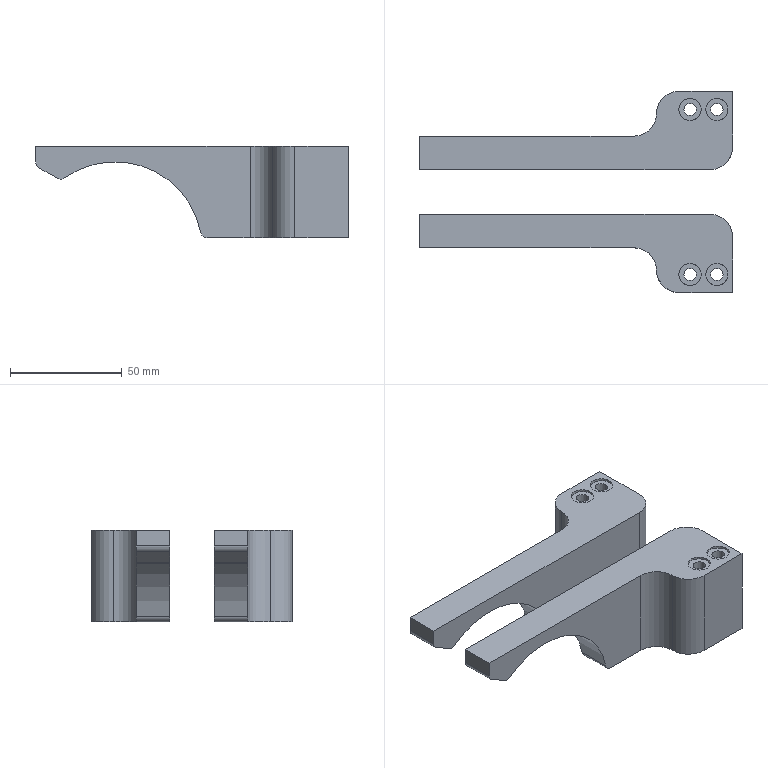NC program | NX | posted with a generic post | part box 140 x 90 x 41 mm
Lines 43 to 1092 of 28919:
(ADAPTIVE_MILLING , TOOL : D12C)
N72 T12 M6
N74 G54
N76 G17 G0 G90 X84.203 Y-7.467 S9500 M3
N78 G43 Z30. H12
N80 Z-17.5
N82 G94 G1 Z-20.5 F1000.
N84 X82.519 Y-6.874 F3000.
N86 G3 X81.036 Y-7.467 R1.218
N88 X80.297 Y-10.773 R9.606
N90 X80.002 Y-19.69 R131.632
N92 G2 X76.897 Y-24.615 R7.1
N94 X70.842 Y-26.888 R14.21
N96 X61.567 Y-27.447 R65.362
N98 G1 X60.442 Y-27.459
N100 X59.092 Y-27.468
N102 X57.517 Y-27.475
N104 X55.267 Y-27.481
N106 X51.817 Y-27.485
N108 X44.242 Y-27.486
N110 X-71.708 Y-27.483
N112 X-71.783
N114 X-71.858 Y-27.481
N116 X-72.007 Y-27.473
N118 X-72.082 Y-27.468
N120 G2 X-77.095 Y-24.379 R7.057
N122 X-79.394 Y-18.256 R14.245
N124 X-79.942 Y-9.431 R62.966
N126 G1 X-79.955 Y-8.306
N128 X-79.965 Y-7.106
N130 X-79.973 Y-5.606
N132 X-79.979 Y-3.581
N134 X-79.984 Y-0.656
N136 X-79.986 Y4.744
N138 G2 X-79.956 Y19.743 R731.547
N140 X-76.746 Y24.687 R7.169
N142 X-70.521 Y26.929 R14.668
N144 X-61.843 Y27.44 R66.663
N146 G1 X-60.793 Y27.451
N148 X-59.518 Y27.462
N150 X-57.943 Y27.47
N152 X-55.918 Y27.476
N154 X-52.918 Y27.48
N156 X-47.218 Y27.483
N158 X44.582 Y27.484
N160 X45.332 Y27.487
N162 X46.232 Y27.488
N164 X46.682
N166 X47.507 Y27.491
N168 X48.707 Y27.49
N170 X49.382 Y27.492
N172 X50.582
N174 X51.557 Y27.494
N176 X52.307
N178 X53.657 Y27.495
N180 X54.107 Y27.496
N182 X54.932 Y27.494
N184 X56.057 Y27.496
N186 X56.807 Y27.495
N188 X58.007 Y27.496
N190 X58.907 Y27.494
N192 X59.657 Y27.495
N194 X60.932 Y27.493
N196 X61.382
N198 X62.207 Y27.495
N200 X63.332 Y27.493
N202 X64.082 Y27.495
N204 X65.357 Y27.493
N206 G2 X72.33 Y27.454 R153.694
N208 X77.24 Y24.187 R7.229
N210 X79.455 Y17.873 R14.887
N212 X79.951 Y8.518 R73.908
N214 X79.941 Y-4.456 R389.185
N216 G3 X79.221 Y-12.674 R226.057
N218 G2 X79.02 Y-17.017 R73.793
N220 X74.352 Y-23.663 R9.401
N222 X67.403 Y-25.901 R18.272
N224 X56.849 Y-26.44 R86.916
N226 G1 X55.574 Y-26.45
N228 X53.999 Y-26.459
N230 X51.974 Y-26.466
N232 X49.124 Y-26.471
N234 X44.399 Y-26.474
N236 X28.949 Y-26.475
N238 X-68.326 Y-26.472
N240 X-68.476 Y-26.471
N242 X-68.701 Y-26.463
N244 X-68.851 Y-26.456
N246 G2 X-75.934 Y-22.12 R9.114
N248 X-78.359 Y-15.085 R17.36
N250 X-78.923 Y-5.659 R73.598
N252 G1 X-78.936 Y-4.609
N254 X-78.947 Y-3.409
N256 X-78.957 Y-1.834
N258 X-78.964 Y0.041
N260 X-78.97 Y2.591
N262 X-78.974 Y6.491
N264 G2 X-78.94 Y16.615 R387.568
N266 X-74.588 Y23.454 R9.146
N268 X-67.547 Y25.863 R17.473
N270 X-57.67 Y26.426 R77.667
N272 G1 X-56.695 Y26.437
N274 X-55.345 Y26.448
N276 X-53.695 Y26.456
N278 X-51.595 Y26.463
N280 X-48.67 Y26.468
N282 X-43.57 Y26.471
N284 X-21.37 Y26.472
N286 X41.18
N288 X42.305 Y26.479
N290 X43.355
N292 X44.33 Y26.484
N294 X45.605 Y26.483
N296 X46.355 Y26.486
N298 X47.33 Y26.487
N300 X47.705
N302 X48.605 Y26.49
N304 X49.73 Y26.489
N306 X50.78 Y26.493
N308 X51.905 Y26.492
N310 X52.88 Y26.494
N312 X53.78 Y26.493
N314 X54.905 Y26.496
N316 X55.955 Y26.494
N318 X57.005 Y26.496
N320 X58.13 Y26.493
N322 X59.255 Y26.495
N324 X60.08 Y26.494
N326 X60.98 Y26.495
N328 X61.355
N330 X62.18 Y26.494
N332 G2 X69.154 Y26.454 R208.519
N334 X75.977 Y22.075 R9.16
N336 X78.357 Y15.101 R17.532
N338 X78.932 Y4.775 R79.803
N340 X78.813 Y-4.596 R113.198
N342 G3 X78.147 Y-14.323 R772.732
N344 G2 X72.411 Y-22.625 R10.832
N346 X64.914 Y-24.877 R20.889
N348 X54.359 Y-25.419 R93.029
N350 G1 X53.159 Y-25.431
N352 X51.734 Y-25.441
N354 X49.934 Y-25.449
N356 X47.684 Y-25.456
N358 X44.384 Y-25.46
N360 X38.609 Y-25.463
N362 X-0.091 Y-25.462
N364 X-65.491 Y-25.46
N366 X-65.791 Y-25.457
N368 X-66.016 Y-25.451
N370 X-66.241 Y-25.441
N372 G2 X-72.322 Y-23.181 R10.254
N374 X-75.927 Y-19.196 R6.416
N376 X-77.65 Y-10.166 R32.289
N378 X-77.954 Y3.703 R225.891
N380 X-77.925 Y14.052 R391.638
N382 X-72.524 Y22.469 R10.509
N384 X-64.844 Y24.866 R20.314
N386 X-54.44 Y25.413 R90.966
N388 G1 X-53.24 Y25.425
N390 X-51.815 Y25.436
N392 X-50.09 Y25.445
N394 X-47.84 Y25.452
N396 X-44.69 Y25.457
N398 X-39.29 Y25.459
N400 X-15.59 Y25.46
N402 X37.81 Y25.461
N404 X38.485 Y25.464
N406 X39.835 Y25.468
N408 X40.51 Y25.469
N410 X41.26 Y25.473
N412 X42.235 Y25.474
N414 X42.685 Y25.475
N416 X43.36 Y25.478
N418 X44.41 Y25.479
N420 X45.16 Y25.482
N422 X45.76 Y25.484
N424 X46.585
N426 X47.785 Y25.488
N428 X48.91 Y25.487
N430 X49.735 Y25.49
N432 X50.785
N434 X51.235
N436 X51.985 Y25.492
N438 X52.96 Y25.491
N440 X53.485 Y25.492
N442 X54.085 Y25.493
N444 X55.285 Y25.492
N446 X56.185 Y25.494
N448 X57.085 Y25.493
N450 G2 X66.609 Y25.447 R290.876
N452 X72.375 Y23.162 R10.225
N454 X75.927 Y19.196 R6.438
N456 X77.619 Y10.54 R31.649
N458 X77.503 Y-8.492 R129.148
N460 X76.984 Y-13.709 R31.363
N462 X70.481 Y-21.7 R12.003
N464 X62.42 Y-23.899 R23.823
N466 X50.887 Y-24.414 R113.709
N468 G1 X49.462 Y-24.425
N470 X47.737 Y-24.434
N472 X45.562 Y-24.442
N474 X42.637 Y-24.447
N476 X37.987 Y-24.451
N478 X26.287 Y-24.452
N480 X-62.963 Y-24.449
N482 X-63.263 Y-24.446
N484 X-63.488 Y-24.442
N486 X-63.788 Y-24.434
N488 G2 X-68.052 Y-23.662 R14.863
N490 X-71.435 Y-23.472 R19.024
N492 G1 X-72.497 Y-23.101
N494 G2 X-75.564 Y-20.101 R6.355
N496 X-76.15 Y-16.64 R7.644
N498 X-76.933 Y3.513 R227.343
N500 X-76.896 Y11.987 R202.597
N502 X-70.759 Y21.434 R11.503
N504 X-62.836 Y23.82 R21.994
N506 X-51.607 Y24.401 R97.353
N508 G1 X-50.407 Y24.413
N510 X-48.907 Y24.424
N512 X-47.182 Y24.433
N514 X-45.007 Y24.439
N516 X-41.857 Y24.445
N518 X-36.757 Y24.448
N520 X-20.407 Y24.449
N522 X34.493
N524 X35.318 Y24.454
N526 X36.143 Y24.455
N528 X36.593 Y24.456
N530 X37.268 Y24.459
N532 X38.543 Y24.462
N534 X39.293 Y24.466
N536 X40.493 Y24.467
N538 X41.168 Y24.471
N540 X42.293 Y24.472
N542 X42.968 Y24.475
N544 X44.018 Y24.477
N546 X44.543 Y24.478
N548 X45.068 Y24.48
N550 X46.043 Y24.481
N552 X46.418
N554 X47.243 Y24.485
N556 X48.443
N558 X49.268 Y24.488
N560 X50.318 Y24.487
N562 X51.293 Y24.49
N564 X52.343 Y24.489
N566 X53.168 Y24.491
N568 X54.068
N570 X54.593
N572 G2 X64.416 Y24.436 R271.367
N574 X68.15 Y23.66 R15.7
N576 X71.435 Y23.472 R18.018
N578 G1 X72.497 Y23.101
N580 G3 X69.965 Y23.65 R7.108
N582 G1 X68.243
N584 G3 X51.898 Y23.888 R308.852
N586 G1 X50.923 Y23.885
N588 X49.648 Y23.887
N590 X48.823 Y23.884
N592 X47.698 Y23.885
N594 X46.348 Y23.88
N596 X45.748
N598 X44.023 Y23.874
N600 X43.423
N602 X42.898 Y23.872
N604 X41.698 Y23.871
N606 X40.873 Y23.868
N608 X40.198 Y23.866
N610 X39.673
N612 X39.148 Y23.864
N614 X37.573 Y23.862
N616 X37.123 Y23.859
N618 X34.123 Y23.857
N620 X23.473 Y23.855
N622 X4.198
N624 X3.898 Y23.854
N626 X-34.577
N628 X-34.952 Y23.852
N630 G3 X-56.176 Y23.685 R749.437
N632 X-65.4 Y22.633 R46.746
N634 X-72.288 Y19.16 R15.199
N636 X-75.81 Y12.195 R12.073
N638 X-76.301 Y3.819 R52.759
N640 X-76.15 Y-6.918 R367.334
N642 G1 Y-16.668
N644 Y-2.535
N646 X-76.146 Y-2.465
N648 G2 X-75.689 Y0.484 R38.279
N650 G3 X-75.204 Y7.816 R154.513
N652 G2 X-73.874 Y14.017 R18.203
N654 X-67.184 Y20.384 R12.794
N656 X-58.901 Y22.35 R26.994
N658 X-46.613 Y22.805 R141.362
N660 G1 X-44.963 Y22.816
N662 X-42.938 Y22.826
N664 X-41.288 Y22.832
N666 X-40.689 Y22.836
N668 X-39.414 Y22.841
N670 X-37.989 Y22.843
N672 X-37.314 Y22.846
N674 X-36.264 Y22.847
N676 X-35.739 Y22.848
N678 X-35.064 Y22.85
N680 X-34.239
N682 X-33.114 Y22.853
N684 X-32.139 Y22.851
N686 X-31.389 Y22.853
N688 X-30.264 Y22.852
N690 X-29.289 Y22.854
N692 X-28.539 Y22.853
N694 X-27.564 Y22.854
N696 X-26.814 Y22.853
N698 X-25.839 Y22.854
N700 X-24.864 Y22.852
N702 X-23.889 Y22.855
N704 X-22.839 Y22.853
N706 X-22.014 Y22.854
N708 X-20.814 Y22.853
N710 X-19.839 Y22.855
N712 X-18.864 Y22.853
N714 X-18.039 Y22.854
N716 X-16.914 Y22.853
N718 X-16.014 Y22.855
N720 X-14.964 Y22.853
N722 X-14.289 Y22.854
N724 X-13.314 Y22.853
N726 X-12.939 Y22.852
N728 X-12.189 Y22.854
N730 X-11.064 Y22.853
N732 X-10.089 Y22.855
N734 X-9.339 Y22.853
N736 X-8.289 Y22.855
N738 X-7.239 Y22.852
N740 X-6.414 Y22.854
N742 X-5.289 Y22.853
N744 X-4.464 Y22.854
N746 X-3.339 Y22.853
N748 X-2.439 Y22.854
N750 X-1.389 Y22.853
N752 X-0.714 Y22.854
N754 X0.261 Y22.853
N756 X0.636 Y22.852
N758 X1.686 Y22.855
N760 X2.436 Y22.854
N762 X3.411 Y22.855
N764 X4.161 Y22.854
N766 X5.136 Y22.856
N768 X6.111 Y22.854
N770 X7.086 Y22.856
N772 X7.911 Y22.854
N774 X9.036 Y22.856
N776 X9.936 Y22.855
N778 X10.911 Y22.856
N780 X11.811 Y22.855
N782 X12.861 Y22.857
N784 X13.536 Y22.855
N786 X14.511 Y22.857
N788 X14.886
N790 X15.636 Y22.856
N792 X16.761 Y22.857
N794 X17.736 Y22.855
N796 X18.486 Y22.856
N798 X19.536 Y22.855
N800 X20.586 Y22.857
N802 X21.486 Y22.855
N804 X22.386 Y22.856
N806 X23.286 Y22.855
N808 X24.261 Y22.857
N810 X25.311 Y22.854
N812 X26.211 Y22.856
N814 X27.336 Y22.854
N816 X28.161 Y22.856
N818 X29.136 Y22.855
N820 X29.961 Y22.856
N822 X30.936 Y22.855
N824 X31.686 Y22.857
N826 X32.736 Y22.856
N828 X33.486 Y22.857
N830 X34.536
N832 X35.286 Y22.859
N834 X36.411
N836 X37.536 Y22.864
N838 X38.286
N840 X39.261 Y22.867
N842 X40.011
N844 X40.911 Y22.87
N846 X40.986 Y22.872
N848 X41.061 Y22.878
N850 X41.135 Y22.89
N852 X43.425 Y23.44
N854 X43.523 Y23.455
N856 X45.975 Y23.648
N858 X46.025 Y23.65
N860 X67.85
N862 G3 X68.674 Y25.722 R1.201
N864 X68.042 Y26.058 Z-20.47 R1.681
N866 G1 X66.469 Y26.642 Z-20.4
N868 X64.309 Y27.434
N870 X64.031 Y27.468
N872 X43.835 Y27.566
N874 G3 X42.658 Y26.628 R1.208
N876 G1 X42.597 Y26.355
N878 X42.075 Y24.013 Z-20.5
N880 G2 X41.641 Y23.15 R1.418
N882 X41.135 Y22.89 R1.334
N884 X36.953 Y22.36 R16.121
N886 X15.504 Y22.256 R921.472
N888 G1 X13.854 Y22.254
N890 X13.329
N892 X12.279 Y22.252
N894 X11.754 Y22.253
N896 X11.079 Y22.254
N898 X10.254 Y22.253
N900 X9.804
N902 X9.129 Y22.254
N904 X8.229 Y22.253
N906 X7.779
N908 X6.954 Y22.252
N910 X6.129 Y22.254
N912 X4.629 Y22.252
N914 X4.029 Y22.254
N916 X3.129 Y22.252
N918 X2.604 Y22.253
N920 X1.929 Y22.252
N922 X1.404
N924 X0.954
N926 X0.354 Y22.254
N928 X-1.221 Y22.251
N930 X-2.196 Y22.253
N932 X-2.946 Y22.252
N934 X-3.396 Y22.253
N936 X-4.971 Y22.251
N938 X-5.946 Y22.253
N940 X-6.471
N942 X-8.871 Y22.251
N944 X-9.021
N946 X-9.846 Y22.253
N948 X-10.596 Y22.252
N950 X-11.046
N952 X-11.796 Y22.251
N954 X-12.246 Y22.252
N956 X-12.696
N958 X-13.296 Y22.254
N960 X-14.946 Y22.251
N962 X-15.771 Y22.253
N964 X-16.521 Y22.252
N966 X-17.196 Y22.254
N968 X-18.246 Y22.252
N970 X-19.746 Y22.255
N972 X-20.196 Y22.254
N974 X-21.246 Y22.256
N976 X-22.071 Y22.254
N978 X-23.796 Y22.256
N980 X-24.471 Y22.254
N982 X-24.921 Y22.255
N984 X-25.446 Y22.253
N986 X-25.971 Y22.254
N988 X-26.346
N990 X-27.171 Y22.255
N992 X-27.621 Y22.254
N994 X-28.296
N996 X-29.121 Y22.255
N998 X-29.571 Y22.254
N1000 X-30.471 Y22.255
N1002 X-32.046 Y22.251
N1004 G3 X-54.019 Y22.042 R682.357
N1006 X-63.307 Y20.902 R45.364
N1008 X-70.38 Y17.153 R15.315
N1010 X-74.014 Y10.046 R13.766
N1012 X-74.842 Y3.126 R56.874
N1014 G2 X-75.147 Y0.825 R13.785
N1016 G3 X-75.972 Y-1.065 R6.947
N1018 G1 X-75.564 Y0.101
N1020 X-75.503 Y0.228
N1022 X-75.186 Y0.733
N1024 G3 X-74.128 Y3.757 R8.235
N1026 G2 X-72.944 Y9.636 R71.263
N1028 X-64.629 Y18.87 R13.679
N1030 X-56.169 Y20.753 R29.149
N1032 X-42.755 Y21.201 R166.238
N1034 G1 X-40.355 Y21.216
N1036 X-37.655 Y21.229
N1038 X-34.955 Y21.237
N1040 X-32.255 Y21.242
N1042 X-30.38 Y21.243
N1044 X-29.78 Y21.246
N1046 X-28.055 Y21.249
N1048 X-26.405
N1050 X-25.28 Y21.247
N1052 X-24.605 Y21.249
N1054 X-22.655 Y21.252
N1056 X-20.705 Y21.25
N1058 X-19.655 Y21.248
N1060 X-18.83 Y21.251
N1062 X-17.93 Y21.25
N1064 X-17.405
N1066 X-16.505 Y21.253
N1068 X-15.53 Y21.251
N1070 X-14.33 Y21.253
N1072 X-13.43 Y21.251
N1074 X-12.605 Y21.253
N1076 X-11.63 Y21.251
N1078 X-10.73 Y21.253
N1080 X-9.455 Y21.25
N1082 X-8.78 Y21.252
N1084 X-7.13 Y21.251
N1086 X-6.08 Y21.249
N1088 X-5.105 Y21.252
N1090 X-4.205 Y21.251
N1092 X-3.23 Y21.253
N1094 X-2.78
N1096 X-1.805 Y21.252
N1098 X-0.68 Y21.254
N1100 X0.145 Y21.252
N1102 X1.345 Y21.254
N1104 X2.095 Y21.253
N1106 X3.22 Y21.254
N1108 X4.27 Y21.252
N1110 X5.095 Y21.254
N1112 X6.07 Y21.252
N1114 X6.67 Y21.253
N1116 X7.87 Y21.252
N1118 X8.47 Y21.251
N1120 X9.145 Y21.252
N1122 X10.345 Y21.251
N1124 X10.795
N1126 X11.845 Y21.254
N1128 X13.27 Y21.251
N1130 X14.245 Y21.254
N1132 X15.07 Y21.253
N1134 X16.195 Y21.255
N1136 X17.17 Y21.254
N1138 X18.37 Y21.257
N1140 X19.195 Y21.255
N1142 X20.395 Y21.258
N1144 X21.145 Y21.257
N1146 X22.195 Y21.259
N1148 X22.795 Y21.261
N1150 X23.62 Y21.259
N1152 X24.52 Y21.261
N1154 X25.12 Y21.263
N1156 G3 X37.192 Y21.434 R239.005
N1158 X38.714 Y21.909 R2.384
N1160 G1 X40.964 Y22.841
N1162 X38.714 Y21.909
N1164 X38.626 Y21.864
N1166 X38.225 Y21.618
N1168 G2 X35.849 Y20.993 R6.072
N1170 X26.633 Y20.679 R91.94
N1172 G1 X24.458 Y20.67
N1174 X22.283 Y20.665
N1176 X21.683
N1178 X21.083 Y20.663
N1180 X17.483 Y20.658
N1182 X15.533 Y20.653
N1184 X14.558 Y20.655
N1186 X13.358 Y20.652
N1188 X11.483 Y20.654
N1190 X10.733 Y20.652
N1192 X9.983 Y20.654
N1194 X9.458 Y20.653
N1196 X9.008 Y20.654
N1198 X8.183 Y20.652
N1200 X6.533 Y20.65
N1202 X6.083 Y20.651
N1204 X2.033 Y20.649
N1206 X1.583 Y20.65
N1208 X0.683 Y20.649
N1210 X-0.517 Y20.652
N1212 X-1.342 Y20.65
N1214 X-2.317 Y20.652
N1216 X-3.892 Y20.649
N1218 X-5.542 Y20.652
N1220 X-6.292 Y20.651
N1222 X-6.667 Y20.652
N1224 X-7.192 Y20.651
N1226 X-8.542 Y20.653
N1228 X-10.117 Y20.655
N1230 X-11.167 Y20.652
N1232 X-11.842 Y20.654
N1234 X-12.442 Y20.653
N1236 X-12.892
N1238 X-13.267 Y20.652
N1240 X-14.017 Y20.653
N1242 X-14.692 Y20.651
N1244 X-15.142 Y20.652
N1246 X-15.442 Y20.651
N1248 X-16.417 Y20.653
N1250 X-16.942 Y20.651
N1252 X-21.142 Y20.655
N1254 X-22.042 Y20.652
N1256 X-22.417
N1258 X-23.017 Y20.65
N1260 X-23.767 Y20.651
N1262 X-24.142 Y20.65
N1264 X-25.192 Y20.652
N1266 G3 X-50.69 Y20.451 R973.861
N1268 X-60.371 Y19.418 R52.975
N1270 X-67.888 Y15.866 R17.09
N1272 X-72.279 Y8.667 R14.978
N1274 X-73.715 Y3.074 R538.158
N1276 G2 X-74.758 Y1.385 R2.846
N1278 G1 X-74.846 Y1.274
N1280 X-75.006 Y1.02
N1282 X-74.846 Y1.274
N1284 X-74.758 Y1.385
N1286 X-74.203 Y1.939
N1288 G3 X-72.848 Y4.161 R5.854
N1290 G2 X-70.941 Y9.211 R114.325
N1292 X-61.841 Y17.502 R15.242
N1294 X-52.806 Y19.216 R34.03
N1296 X-37.739 Y19.608 R224.519
N1298 G1 X-34.064 Y19.622
N1300 X-30.239 Y19.632
N1302 X-26.414 Y19.638
N1304 X-25.064 Y19.639
N1306 X-24.239 Y19.644
N1308 X-23.339 Y19.645
N1310 X-20.189 Y19.643
N1312 X-19.364 Y19.646
N1314 X-18.389 Y19.647
N1316 X-17.864 Y19.646
N1318 X-16.889 Y19.65
N1320 X-16.139 Y19.649
N1322 X-14.939 Y19.652
N1324 X-14.264
N1326 X-13.814 Y19.651
N1328 X-12.764 Y19.654
N1330 X-11.939 Y19.652
N1332 X-10.964 Y19.654
N1334 X-10.064 Y19.651
N1336 X-8.789 Y19.654
N1338 X-7.439 Y19.65
N1340 X-6.014 Y19.653
N1342 X-5.189 Y19.651
N1344 X-3.914 Y19.653
N1346 X-2.489 Y19.649
N1348 X-1.814 Y19.65
N1350 X-0.464 Y19.649
N1352 X0.136 Y19.648
N1354 X0.886 Y19.649
N1356 X1.861
N1358 X2.686 Y19.65
N1360 X3.736 Y19.649
N1362 X4.636 Y19.651
N1364 X5.611 Y19.65
N1366 X6.361 Y19.652
N1368 X7.411 Y19.651
N1370 X8.536 Y19.654
N1372 X9.736 Y19.651
N1374 X11.086 Y19.654
N1376 X11.836 Y19.653
N1378 X12.886 Y19.655
N1380 X13.711 Y19.657
N1382 X14.311 Y19.656
N1384 G3 X32.384 Y19.804 R607.162
N1386 X35.957 Y20.188 R20.691
N1388 G1 X38.148 Y21.571
N1390 X36.55 Y20.592
N1392 X36.47 Y20.533
N1394 X36.241 Y20.338
N1396 G2 X34.441 Y19.645 R3.956
N1398 X28.093 Y19.146 R38.944
N1400 X7.243 Y19.054 R989.262
N1402 G1 X5.968 Y19.051
N1404 X5.368 Y19.052
N1406 X4.093 Y19.049
N1408 X3.118 Y19.05
N1410 X2.668
N1412 X1.693 Y19.051
N1414 X1.243 Y19.05
N1416 X0.493 Y19.052
N1418 X-0.257 Y19.05
N1420 X-1.532 Y19.053
N1422 X-2.282 Y19.051
N1424 X-3.632 Y19.054
N1426 X-4.157 Y19.053
N1428 X-4.682
N1430 X-5.132 Y19.052
N1432 X-6.332 Y19.054
N1434 X-7.082 Y19.052
N1436 X-8.732 Y19.055
N1438 X-9.707 Y19.053
N1440 X-10.157 Y19.054
N1442 X-10.982 Y19.052
N1444 X-12.407 Y19.054
N1446 X-12.932 Y19.052
N1448 X-13.532 Y19.053
N1450 X-14.132 Y19.051
N1452 X-15.257 Y19.049
N1454 X-16.982 Y19.05
N1456 X-17.807 Y19.047
N1458 X-20.957 Y19.05
N1460 X-23.507 Y19.041
N1462 X-24.332
N1464 X-25.082 Y19.039
N1466 G3 X-48.255 Y18.837 R859.304
N1468 X-58.162 Y17.795 R56.266
N1470 X-66.17 Y14.062 R18.243
N1472 X-70.649 Y7.758 R17.376
N1474 G2 X-72.677 Y3.328 R52.45
N1476 X-73.774 Y2.346 R2.464
N1478 G1 X-73.885 Y2.258
N1480 X-73.991 Y2.152
N1482 X-73.885 Y2.258
N1484 X-73.774 Y2.346
N1486 X-73.157 Y2.734
N1488 G3 X-71.489 Y4.527 R5.041
N1490 G2 X-68.848 Y8.976 R201.268
N1492 X-58.934 Y16.187 R17.555
N1494 X-49.771 Y17.657 R40.671
N1496 X-33.277 Y18.005 R291.552
N1498 G1 X-30.502 Y18.015
N1500 X-29.977 Y18.019
N1502 X-28.553 Y18.026
N1504 X-27.203 Y18.028
N1506 X-26.678 Y18.029
N1508 X-25.853 Y18.033
N1510 X-24.728 Y18.035
N1512 X-24.053 Y18.039
N1514 X-23.003 Y18.041
N1516 X-22.328
N1518 X-21.653 Y18.043
N1520 X-20.528 Y18.044
N1522 X-19.778 Y18.046
N1524 X-18.653 Y18.045
N1526 X-17.528 Y18.049
N1528 X-16.853
N1530 X-15.653 Y18.052
N1532 X-15.128
N1534 X-14.153 Y18.05
N1536 X-13.403 Y18.052
N1538 X-12.203 Y18.051
N1540 X-11.228 Y18.053
N1542 X-10.178 Y18.052
N1544 X-9.128 Y18.054
N1546 X-8.378 Y18.053
N1548 X-7.178 Y18.054
N1550 X-6.578 Y18.055
N1552 X-5.528 Y18.052
N1554 X-4.478 Y18.054
N1556 X-3.353 Y18.051
N1558 X-2.603 Y18.052
N1560 X-1.328 Y18.05
N1562 X-0.728 Y18.049
N1564 X0.172 Y18.051
N1566 X1.147 Y18.049
N1568 X2.272 Y18.052
N1570 X3.097 Y18.05
N1572 X4.222 Y18.052
N1574 X4.972
N1576 X6.022 Y18.054
N1578 X7.147 Y18.052
N1580 X7.897 Y18.054
N1582 X9.022
N1584 X9.472
N1586 X10.522 Y18.057
N1588 X11.572 Y18.056
N1590 X12.472 Y18.059
N1592 X13.672 Y18.058
N1594 X14.347 Y18.06
N1596 X15.622 Y18.061
N1598 X16.747 Y18.066
N1600 X17.422
N1602 G3 X30.918 Y18.313 R244.579
N1604 X34.464 Y18.881 R16.422
N1606 X36.129 Y20.243 R14.787
N1608 G1 X34.704 Y19.025
N1610 G2 X32.538 Y18.145 R4.727
N1612 X25.372 Y17.559 R41.517
N1614 X4.372 Y17.455 R963.739
N1616 G1 X3.397 Y17.452
N1618 X2.422 Y17.453
N1620 X1.897 Y17.451
N1622 X0.622 Y17.453
N1624 X0.172 Y17.452
N1626 X-0.353 Y17.453
N1628 X-0.953 Y17.452
N1630 X-1.853 Y17.454
N1632 X-3.203 Y17.451
N1634 X-3.803 Y17.453
N1636 X-6.203 Y17.45
N1638 X-6.728 Y17.452
N1640 X-7.628 Y17.45
N1642 X-8.603 Y17.453
N1644 X-9.578 Y17.451
N1646 X-10.403 Y17.45
N1648 X-13.253 Y17.448
N1650 X-16.028 Y17.449
N1652 X-16.628
N1654 X-18.053
N1656 X-18.653 Y17.447
N1658 X-19.103
N1660 X-19.853 Y17.444
N1662 X-20.378
N1664 X-21.878 Y17.443
N1666 X-22.403 Y17.441
N1668 X-23.528 Y17.44
N1670 X-24.353 Y17.436
N1672 X-24.953 Y17.435
N1674 X-25.478 Y17.433
N1676 X-26.153 Y17.432
N1678 X-30.277 Y17.413
N1680 G3 X-48.498 Y17.104 R385.
N1682 X-58.19 Y15.638 R42.681
N1684 X-68.637 Y7.807 R18.31
N1686 G2 X-71.404 Y3.798 R45.861
N1688 X-72.601 Y3.064 R2.091
N1690 G1 X-72.728 Y3.003
N1692 X-72.855 Y2.923
N1694 X-72.728 Y3.003
N1696 X-72.601 Y3.064
N1698 X-72.061 Y3.253
N1700 G3 X-70.033 Y4.747 R4.771
N1702 G2 X-66.585 Y8.803 R329.324
N1704 X-55.79 Y14.921 R20.838
N1706 X-45.306 Y16.17 R54.973
N1708 X-24.683 Y16.427 R648.251
N1710 G1 X-20.333 Y16.446
N1712 X-19.284 Y16.445
N1714 X-18.609 Y16.446
N1716 X-17.334
N1718 X-16.734 Y16.445
N1720 X-16.059 Y16.446
N1722 X-14.784
N1724 X-14.409 Y16.445
N1726 X-13.734 Y16.447
N1728 X-12.684
N1730 X-12.159 Y16.448
N1732 X-11.484 Y16.45
N1734 X-10.509 Y16.449
N1736 X-9.684 Y16.451
N1738 X-8.484 Y16.449
N1740 X-7.734 Y16.451
N1742 X-6.834 Y16.45
N1744 X-6.384 Y16.449
N1746 X-5.259 Y16.452
N1748 X-4.134 Y16.45
N1750 X-3.384 Y16.451
N1752 X-2.184 Y16.45
N1754 X-1.359 Y16.449
N1756 X-0.384 Y16.451
N1758 X0.591 Y16.45
N1760 X1.491 Y16.452
N1762 X2.766 Y16.451
N1764 X3.741 Y16.454
N1766 X4.566 Y16.453
N1768 X5.541 Y16.455
N1770 X6.441 Y16.454
N1772 X7.491 Y16.457
N1774 X8.466 Y16.456
N1776 X9.666 Y16.461
N1778 G3 X27.589 Y16.676 R438.291
N1780 X33.06 Y17.503 R21.508
N1782 X33.661 Y17.843 R2.257
N1784 G1 X34.548 Y18.882
N1786 X34.618 Y18.952
N1788 X34.548 Y18.882
N1790 X33.661 Y17.843
N1792 G2 X31.976 Y16.914 R3.511
N1794 X25.825 Y16.068 R25.655
N1796 X7.677 Y15.86 R493.583
N1798 G1 X4.602 Y15.853
N1800 X4.077 Y15.852
N1802 X3.252 Y15.85
N1804 X1.902 Y15.852
N1806 X1.227 Y15.85
N1808 X-0.048 Y15.853
N1810 X-0.648 Y15.851
N1812 X-1.248 Y15.852
N1814 X-1.698
N1816 X-2.898 Y15.854
N1818 X-3.798 Y15.851
N1820 X-4.698 Y15.852
N1822 X-6.048 Y15.849
N1824 X-6.573 Y15.85
N1826 X-7.173 Y15.849
N1828 X-7.473 Y15.85
N1830 X-8.148 Y15.849
N1832 X-8.673 Y15.85
N1834 X-10.623 Y15.846
N1836 X-11.298 Y15.847
N1838 X-12.123 Y15.846
N1840 X-12.723 Y15.847
N1842 X-13.473 Y15.845
N1844 X-14.073 Y15.846
N1846 X-14.523
N1848 X-15.273 Y15.847
N1850 X-16.923 Y15.844
N1852 X-18.048 Y15.846
N1854 X-21.723 Y15.834
N1856 X-25.398 Y15.819
N1858 X-27.048 Y15.811
N1860 X-27.573 Y15.81
N1862 G3 X-45.644 Y15.529 R462.834
N1864 X-55.884 Y14.16 R49.841
N1866 X-66.817 Y7.401 R21.703
N1868 G2 X-70.156 Y3.96 R35.374
N1870 X-71.435 Y3.472 R2.115
N1872 G1 X-71.789 Y3.349
N1874 X-71.435 Y3.472
N1876 X-71.298 Y3.504
N1878 X-70.942 Y3.544
N1880 G3 X-68.798 Y4.543 R4.122
N1882 X-64.722 Y8.082 R147.494
N1884 G2 X-52.733 Y13.596 R25.347
N1886 X-41.617 Y14.617 R72.542
N1888 X-20.093 Y14.828 R900.587
N1890 G1 X-15.968 Y14.84
N1892 X-11.843 Y14.848
N1894 X-7.718 Y14.853
N1896 X-3.593
N1898 X0.532 Y14.85
N1900 X1.957 Y14.848
N1902 G3 X24.005 Y15.029 R831.467
N1904 X30.923 Y15.812 R33.369
N1906 X32.575 Y16.49 R4.298
N1908 G2 X33.6 Y17.772 R31.443
N1910 G1 X32.967 Y17.03
N1912 X32.908 Y16.95
N1914 X32.748 Y16.689
N1916 G2 X31.381 Y15.693 R2.563
N1918 X26.032 Y14.626 R18.53
N1920 X13.89 Y14.289 R181.065
N1922 G1 X12.165 Y14.279
N1924 X10.89 Y14.274
N1926 X10.365 Y14.27
N1928 X9.24 Y14.268
N1930 X7.065 Y14.264
N1932 X6.315 Y14.26
N1934 X5.415 Y14.259
N1936 X4.365 Y14.254
N1938 X0.69 Y14.256
N1940 X0.09
N1942 X-0.285 Y14.255
N1944 X-2.085 Y14.257
N1946 X-2.535 Y14.256
N1948 X-3.735 Y14.257
N1950 X-4.26 Y14.255
N1952 X-5.235 Y14.256
N1954 X-5.835 Y14.254
N1956 X-6.585 Y14.255
N1958 X-7.185 Y14.253
N1960 X-7.785 Y14.254
N1962 X-8.535 Y14.251
N1964 X-9.135 Y14.252
N1966 X-10.035 Y14.249
N1968 X-10.485 Y14.25
N1970 X-11.535 Y14.246
N1972 X-11.985 Y14.247
N1974 X-13.635 Y14.241
N1976 X-14.01 Y14.242
N1978 X-26.835 Y14.2
N1980 X-28.185 Y14.19
N1982 X-28.635 Y14.189
N1984 X-34.485 Y14.144
N1986 G3 X-48.268 Y13.57 R154.179
N1988 X-58.293 Y11.166 R33.639
N1990 X-65.496 Y6.483 R28.921
N1992 G2 X-69.172 Y3.776 R21.937
N1994 X-70.035 Y3.646 R2.128
N1996 G1 X-70.706 Y3.57
N1998 X-70.035 Y3.646
N2000 X-69.965 Y3.65
N2002 X-69.661
N2004 G3 X-67.327 Y4.371 R4.466
N2006 X-62.759 Y7.385 R89.711
N2008 G2 X-49.498 Y12.25 R31.197
N2010 X-36.633 Y13.08 R105.543
N2012 G1 X-35.508 Y13.099
N2014 X-34.083 Y13.119
N2016 X-32.283 Y13.14
N2018 X-30.183 Y13.16
N2020 X-28.083 Y13.176
N2022 X-25.983 Y13.189
N2024 X-23.508 Y13.199
N2026 X-10.234 Y13.242
N2028 X-5.134 Y13.258
N2030 X-3.934 Y13.255
N2032 X-2.809 Y13.257
N2034 X-1.984 Y13.256
N2036 X-1.009
N2038 G3 X22.464 Y13.461 R736.502
N2040 X29.745 Y14.348 R33.676
N2042 X31.801 Y15.228 R5.988
N2044 X32.681 Y16.579 R11.157
N2046 G1 X31.976 Y15.428
N2048 G2 X30.436 Y14.286 R3.08
N2050 X24.81 Y13.088 R18.986
N2052 X11.995 Y12.696 R170.914
N2054 G1 X10.27 Y12.685
N2056 X6.97 Y12.669
N2058 X3.82 Y12.658
N2060 X3.295
N2062 X2.47 Y12.656
N2064 X1.495 Y12.657
N2066 X0.445 Y12.655
N2068 X-0.155 Y12.657
N2070 X-1.28 Y12.654
N2072 X-2.405 Y12.657
N2074 X-10.13 Y12.645
N2076 X-10.655 Y12.642
N2078 X-11.555 Y12.64
N2080 X-12.08 Y12.637
N2082 X-12.905 Y12.636
N2084 X-13.43 Y12.633
N2086 X-14.255 Y12.632
N2088 X-14.78 Y12.628
N2090 X-15.605 Y12.627
N2092 X-16.205 Y12.624
N2094 X-17.105 Y12.622
N2096 X-17.705 Y12.619
N2098 G3 X-41.177 Y12.329 R716.833
N2100 X-52.702 Y10.949 R61.279
N2102 X-63.068 Y6.351 R32.205
N2104 G2 X-67.47 Y3.789 R30.674
N2106 G1 X-67.61 Y3.734
N2108 X-67.681 Y3.71
N2110 X-67.753 Y3.689
N2112 X-67.826 Y3.672
N2114 X-67.9 Y3.66
N2116 X-67.974 Y3.651
N2118 X-67.987 Y3.65
N2120 X-69.412
N2122 X-67.987
N2124 G3 X-64.97 Y4.435 R6.477
N2126 G1 X-64.766 Y4.531
N2128 X-64.63 Y4.595
N2130 X-64.293 Y4.759
N2132 X-64.025 Y4.895
N2134 X-63.692 Y5.067
N2136 X-63.427 Y5.207
N2138 X-63.03 Y5.419
N2140 X-62.303 Y5.809
N2142 X-61.509 Y6.233
N2144 X-61.177 Y6.407
N2146 X-60.778 Y6.615
N2148 X-60.376 Y6.818
N2150 X-59.906 Y7.052
N2152 X-59.502 Y7.249
N2154 G2 X-46.404 Y10.838 R39.16
N2156 X-32.626 Y11.505 R147.168
N2158 G1 X-31.201 Y11.524
N2160 X-29.776 Y11.54
N2162 X-27.751 Y11.557
N2164 X-24.376 Y11.579